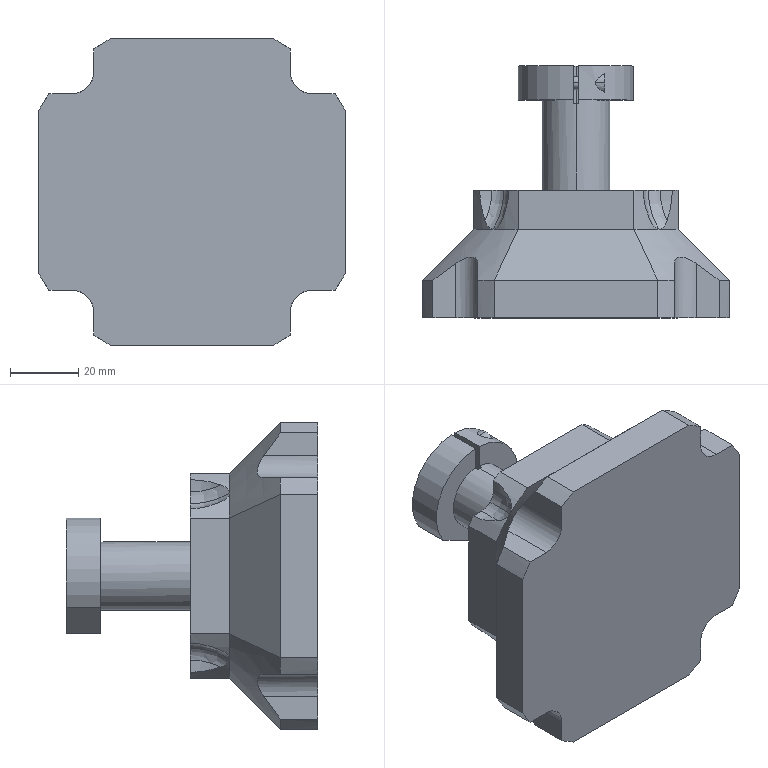Part | STEP file | AB0902-1 | 1 solid | 80 faces | box 90 x 74 x 90 mm | volume 203624 mm3 | cylinder 30 | plane 30 | spline 12 | cone 8 | commonest cylinder face diameters 69 x8 102 x8 13 x4 4 x2 7 x2 16 x2